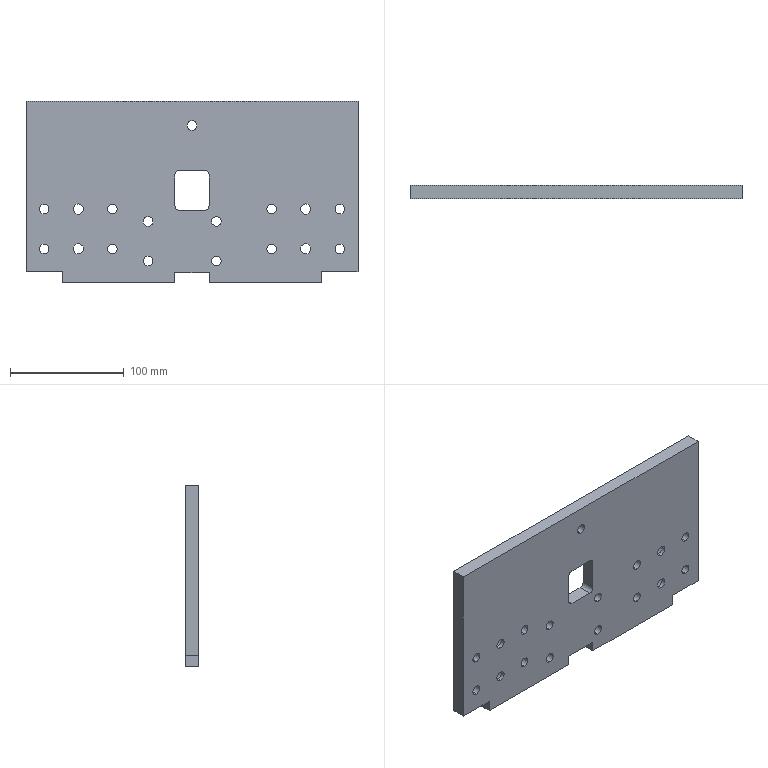Part | STEP file | PN_0017 (fixed block) | 1 solid | 68 faces | box 292 x 12 x 160 mm | volume 521488 mm3 | cylinder 46 | plane 22 | commonest cylinder face diameters 8.5 x26 9 x8 15 x8 8 x4